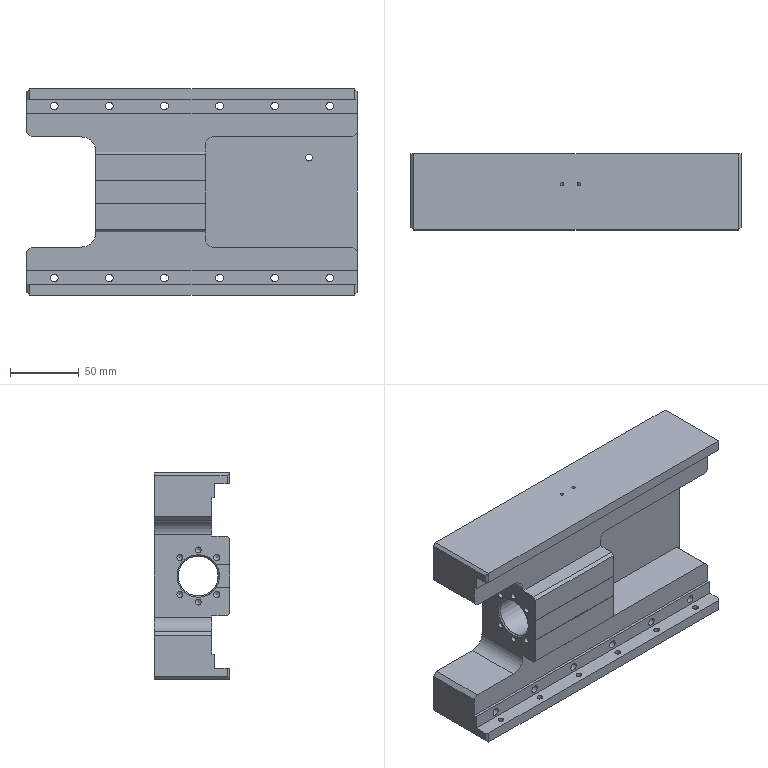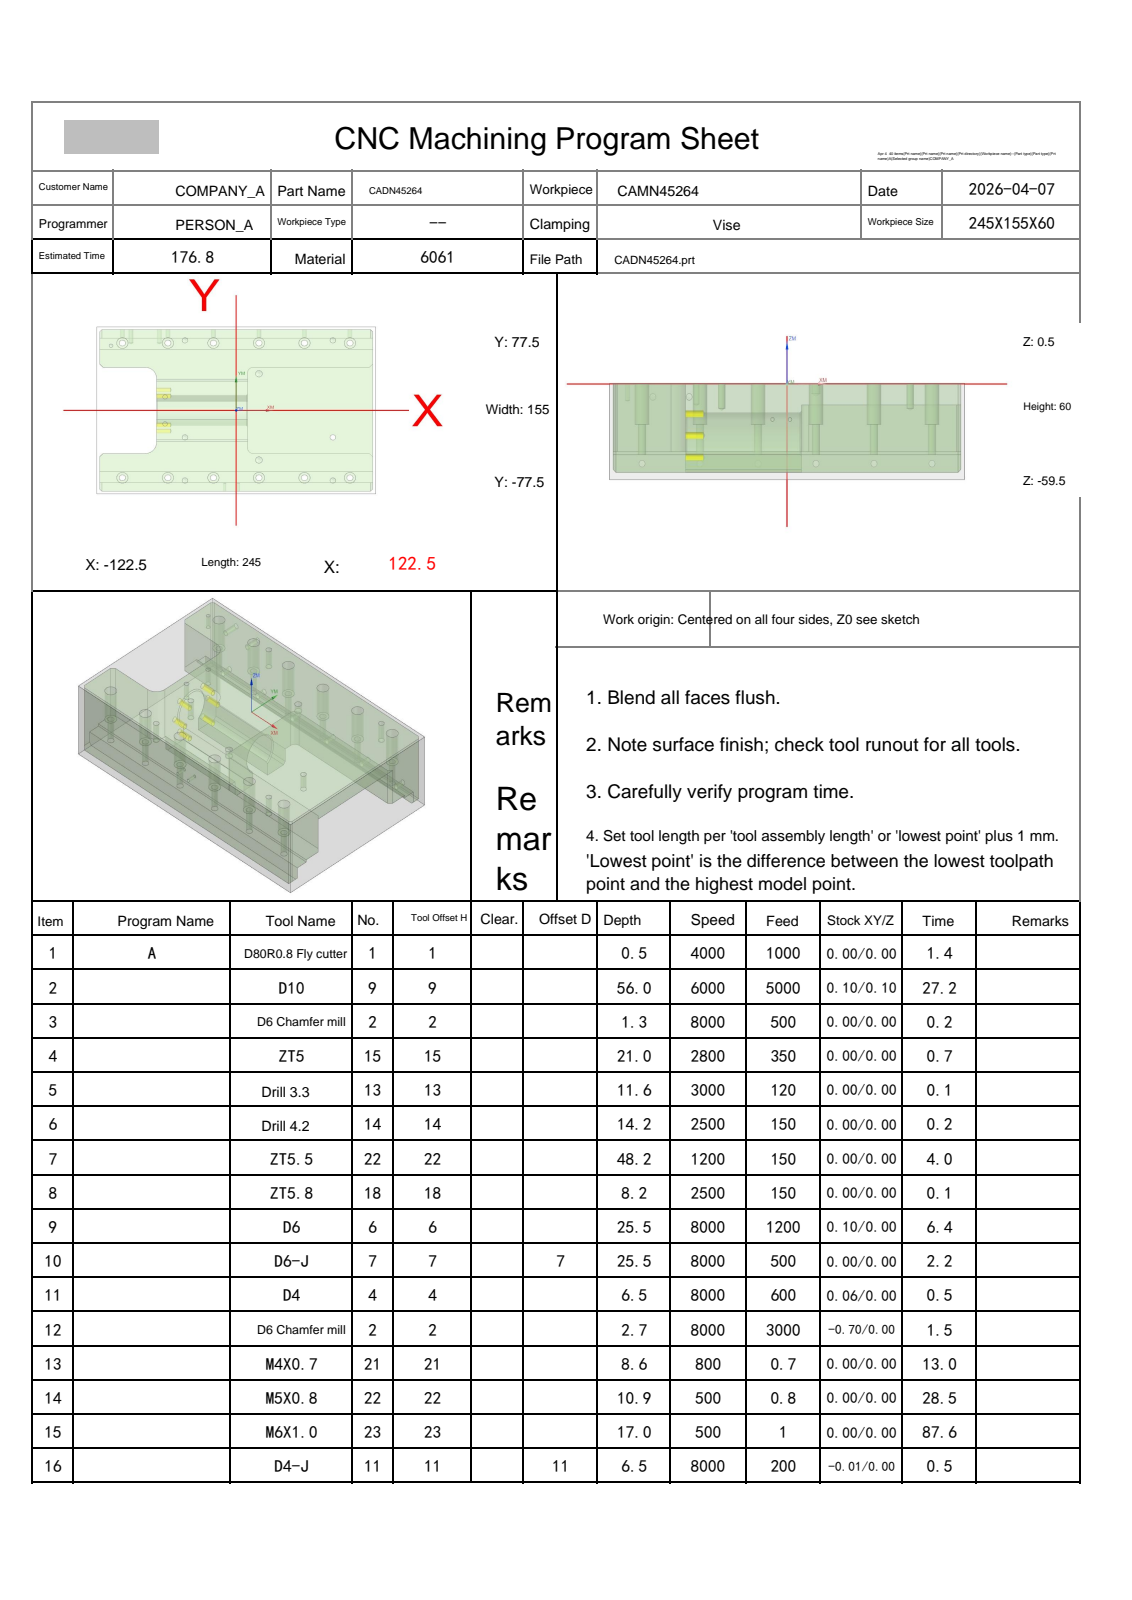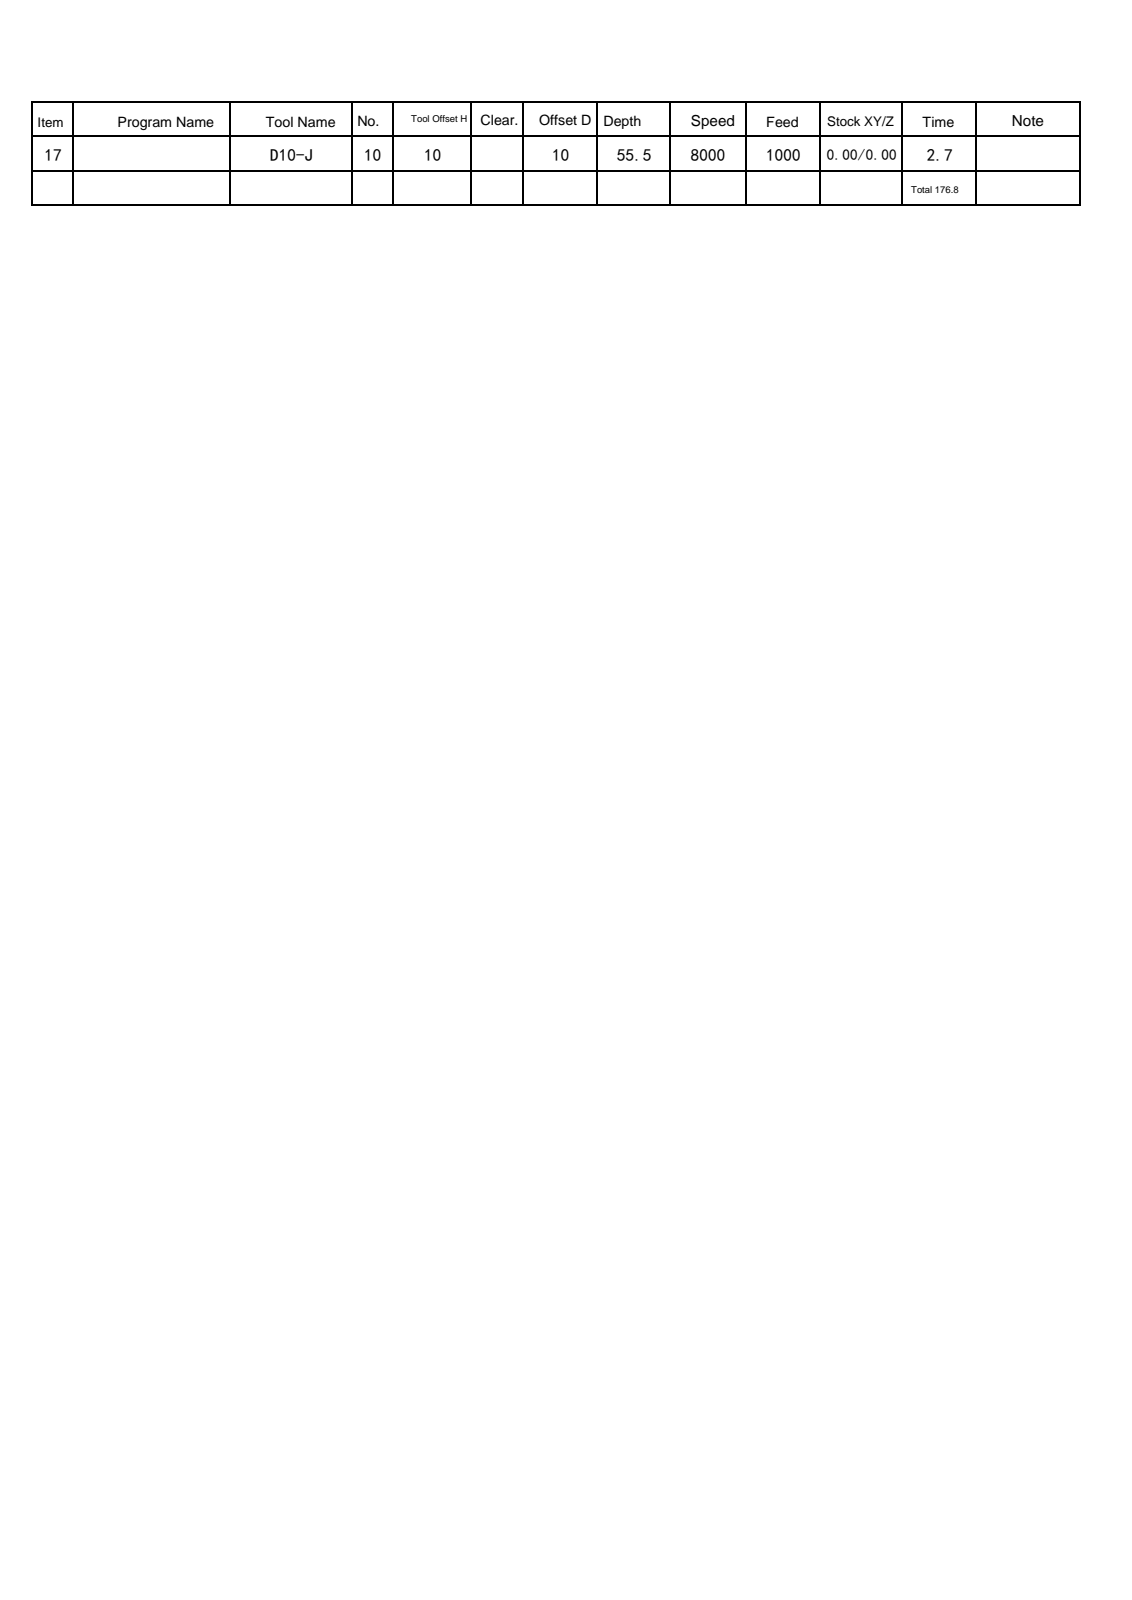NC program | NX | posted by the shop | part box 240 x 55 x 150 mm
Lines 48 to 1046 of 12612:
N2 T09 M06
(D10  D=10. R=0. H=09 ce=0.10 di=0.10)
G00 G90 G54 X-134.5 Y-.734 M03 S6000
G43 H09 Z10.5
M08
Z.603
G01 Z-.597 F5000.
G02 X-129.333 Y1.543 I5.167 J-4.722
X-127.5 Y1.299 I0.0 J-7.
G03 X-123.278 Y.395 I10.5 J38.701
G02 X-122.944 Y0.0 I-.066 J-.395
X-123.278 Y-.395 I-.4 J0.0
G03 X-126.743 Y-1.102 I6.278 J-39.605
X-127.5 Y-2.071 I.243 J-.97
G01 Y-7.652
G03 X-126.8 Y-8.352 I.7 J0.0
X-126.597 Y-8.322 I0.0 J.7
G02 X-117. Y-6.9 I9.597 J-31.678
G01 X-104.096
G03 X-103.1 Y-5.904 I-.004 J1.
G01 Y-2.469
X-103.071 Y-2.414
X-103.13 Y-2.397
X-103.2 Y-2.328
X-103.27 Y-2.296
X-103.247 Y-2.222
G03 X-105.27 Y.1 I-2.496 J-.133
G01 X-119.827 Y2.91
G03 X-120.301 Y2.955 I-.474 J-2.455
X-122.801 Y.455 I0.0 J-2.5
X-120.774 Y-2. I2.5 J0.0
G01 X-106.217 Y-4.81
G03 X-105.743 Y-4.855 I.474 J2.455
X-103.246 Y-2.466 I0.0 J2.5
G01 X-103.216 Y-2.398
X-103.148 Y-2.331
X-103.076 Y-2.293
X-103.1 Y-2.215
Y5.904
G03 X-104.096 Y6.9 I-1. J-.004
G01 X-117.
G02 X-126.796 Y8.383 I0.0 J33.1
X-127.5 Y9.338 I.296 J.955
G01 Y15.203
G02 X-126.9 Y15.803 I.6 J0.0
X-126.678 Y15.761 I0.0 J-.6
G03 X-117. Y13.9 I9.678 J24.239
G01 X-97.096
G02 X-96.1 Y12.904 I-.004 J-1.
G01 Y-12.904
G02 X-97.096 Y-13.9 I-1. J.004
G01 X-117.
G03 X-126.879 Y-15.842 I0.0 J-26.1
X-127.5 Y-16.767 I.379 J-.925
G01 Y-23.143
G03 X-127. Y-23.643 I.5 J0.0
X-126.745 Y-23.573 I0.0 J.5
G02 X-117. Y-20.9 I9.745 J-16.427
G01 X-90.097
G03 X-89.1 Y-19.903 I-.003 J1.
G01 Y19.903
G03 X-90.097 Y20.9 I-1. J-.003
G01 X-117.
G02 X-127.025 Y23.743 I0.0 J19.1
X-127.5 Y24.593 I.525 J.851
G01 Y32.423
G02 X-127.1 Y32.822 I.4 J0.0
X-126.817 Y32.705 I0.0 J-.4
G01 X-125.556 Y31.444
G03 X-117. Y27.9 I8.556 J8.556
G01 X-83.098
G02 X-82.1 Y26.902 I-.002 J-1.
G01 Y-26.902
G02 X-83.098 Y-27.9 I-1. J.002
G01 X-117.
G03 X-125.556 Y-31.444 I0.0 J-12.1
G01 X-126.903 Y-32.791
G03 X-127.195 Y-33.498 I.707 J-.707
X-127.011 Y-34.077 I1. J0.0
G01 X-124.072 Y-38.21
G03 X-123.257 Y-38.631 I.815 J.579
X-122.55 Y-38.338 I0.0 J1.
G01 X-120.606 Y-36.394
G02 X-117. Y-34.9 I3.606 J-3.606
G01 X-80.
G03 X-75.1 Y-30. I0.0 J4.9
G01 Y30.
G03 X-80. Y34.9 I-4.9 J0.0
G01 X-117.
G02 X-120.606 Y36.394 I0.0 J5.1
G01 X-123.606 Y39.394
G02 X-125.1 Y43. I3.606 J3.606
G01 Y73.
G02 X-123.606 Y76.606 I5.1 J0.0
G01 X-121.606 Y78.606
G02 X-118. Y80.1 I3.606 J-3.606
G01 X118.
G02 X121.606 Y78.606 I0.0 J-5.1
G01 X123.606 Y76.606
G02 X125.1 Y73. I-3.606 J-3.606
G01 Y-73.
G02 X123.606 Y-76.606 I-5.1 J0.0
G01 X121.606 Y-78.606
G02 X118. Y-80.1 I-3.606 J3.606
G01 X-118.
G02 X-121.606 Y-78.606 I0.0 J5.1
G01 X-123.606 Y-76.606
G02 X-125.1 Y-73. I3.606 J3.606
G01 Y-43.
G02 X-123.606 Y-39.394 I5.1 J0.0
G01 X-120.606 Y-36.394
G02 X-118.72 Y-35.199 I3.606 J-3.606
X-118.242 Y-35.054 I1.72 J-4.801
G03 X-112.947 Y-28.264 I-1.705 J6.789
X-113.158 Y-26.559 I-7. J0.0
G01 Z.603
G00 Z3.
G01 X-134.5 Y-.734 F6000.
G00 Z.006
G01 Z-1.194 F5000.
G02 X-129.333 Y1.543 I5.167 J-4.722
X-127.5 Y1.299 I0.0 J-7.
G03 X-123.279 Y.395 I10.5 J38.701
G02 X-122.944 Y0.0 I-.066 J-.395
X-123.279 Y-.395 I-.4 J0.0
G03 X-126.743 Y-1.102 I6.279 J-39.605
X-127.5 Y-2.071 I.243 J-.97
G01 Y-7.652
G03 X-126.8 Y-8.352 I.7 J0.0
X-126.597 Y-8.322 I0.0 J.7
G02 X-117. Y-6.9 I9.597 J-31.678
G01 X-104.096
G03 X-103.1 Y-5.904 I-.004 J1.
G01 Y-2.469
X-103.071 Y-2.414
X-103.13 Y-2.397
X-103.2 Y-2.328
X-103.27 Y-2.295
X-103.247 Y-2.222
G03 X-105.27 Y.1 I-2.496 J-.133
G01 X-119.827 Y2.91
G03 X-120.301 Y2.955 I-.474 J-2.455
X-122.801 Y.455 I0.0 J-2.5
X-120.774 Y-2. I2.5 J0.0
G01 X-106.217 Y-4.81
G03 X-105.743 Y-4.855 I.474 J2.455
X-103.246 Y-2.466 I0.0 J2.5
G01 X-103.216 Y-2.398
X-103.148 Y-2.331
X-103.076 Y-2.293
X-103.1 Y-2.215
Y5.904
G03 X-104.096 Y6.9 I-1. J-.004
G01 X-117.
G02 X-126.796 Y8.383 I0.0 J33.1
X-127.5 Y9.338 I.296 J.955
G01 Y15.203
G02 X-126.9 Y15.803 I.6 J0.0
X-126.678 Y15.761 I0.0 J-.6
G03 X-117. Y13.9 I9.678 J24.239
G01 X-97.097
G02 X-96.1 Y12.903 I-.003 J-1.
G01 Y-12.903
G02 X-97.097 Y-13.9 I-1. J.003
G01 X-117.
G03 X-126.879 Y-15.842 I0.0 J-26.1
X-127.5 Y-16.767 I.379 J-.925
G01 Y-23.143
G03 X-127. Y-23.643 I.5 J0.0
X-126.745 Y-23.573 I0.0 J.5
G02 X-117. Y-20.9 I9.745 J-16.427
G01 X-90.098
G03 X-89.1 Y-19.902 I-.002 J1.
G01 Y19.902
G03 X-90.098 Y20.9 I-1. J-.002
G01 X-117.
G02 X-127.025 Y23.743 I0.0 J19.1
X-127.5 Y24.593 I.525 J.851
G01 Y32.423
G02 X-127.1 Y32.822 I.4 J0.0
X-126.817 Y32.705 I0.0 J-.4
G01 X-125.556 Y31.444
G03 X-117. Y27.9 I8.556 J8.556
G01 X-83.099
G02 X-82.1 Y26.901 I-.001 J-1.
G01 Y-26.901
G02 X-83.099 Y-27.9 I-1. J.001
G01 X-117.
G03 X-125.556 Y-31.444 I0.0 J-12.1
G01 X-126.903 Y-32.791
G03 X-127.195 Y-33.498 I.707 J-.707
X-127.011 Y-34.077 I1. J0.0
G01 X-124.072 Y-38.21
G03 X-123.257 Y-38.631 I.815 J.579
X-122.55 Y-38.338 I0.0 J1.
G01 X-120.606 Y-36.394
G02 X-117. Y-34.9 I3.606 J-3.606
G01 X-80.
G03 X-75.1 Y-30. I0.0 J4.9
G01 Y30.
G03 X-80. Y34.9 I-4.9 J0.0
G01 X-117.
G02 X-120.606 Y36.394 I0.0 J5.1
G01 X-123.606 Y39.394
G02 X-125.1 Y43. I3.606 J3.606
G01 Y73.
G02 X-123.606 Y76.606 I5.1 J0.0
G01 X-121.606 Y78.606
G02 X-118. Y80.1 I3.606 J-3.606
G01 X118.
G02 X121.606 Y78.606 I0.0 J-5.1
G01 X123.606 Y76.606
G02 X125.1 Y73. I-3.606 J-3.606
G01 Y-73.
G02 X123.606 Y-76.606 I-5.1 J0.0
G01 X121.606 Y-78.606
G02 X118. Y-80.1 I-3.606 J3.606
G01 X-118.
G02 X-121.606 Y-78.606 I0.0 J5.1
G01 X-123.606 Y-76.606
G02 X-125.1 Y-73. I3.606 J3.606
G01 Y-43.
G02 X-123.606 Y-39.394 I5.1 J0.0
G01 X-120.606 Y-36.394
G02 X-118.72 Y-35.199 I3.606 J-3.606
X-118.242 Y-35.054 I1.72 J-4.801
G03 X-112.947 Y-28.264 I-1.705 J6.789
X-113.158 Y-26.559 I-7. J0.0
G01 Z.006
G00 Z2.403
G01 X-134.5 Y-.734 F6000.
G00 Z-.591
G01 Z-1.791 F5000.
G02 X-129.333 Y1.543 I5.167 J-4.722
X-127.5 Y1.299 I0.0 J-7.
G03 X-123.278 Y.395 I10.5 J38.701
G02 X-122.944 Y0.0 I-.066 J-.395
X-123.278 Y-.395 I-.4 J0.0
G03 X-126.743 Y-1.102 I6.278 J-39.605
X-127.5 Y-2.071 I.243 J-.97
G01 Y-7.652
G03 X-126.8 Y-8.352 I.7 J0.0
X-126.597 Y-8.322 I0.0 J.7
G02 X-117. Y-6.9 I9.597 J-31.678
G01 X-104.096
G03 X-103.1 Y-5.904 I-.004 J1.
G01 Y-2.469
X-103.071 Y-2.414
X-103.13 Y-2.397
X-103.2 Y-2.328
X-103.27 Y-2.296
X-103.247 Y-2.222
G03 X-105.27 Y.1 I-2.496 J-.133
G01 X-119.827 Y2.91
G03 X-120.301 Y2.955 I-.474 J-2.455
X-122.801 Y.455 I0.0 J-2.5
X-120.774 Y-2. I2.5 J0.0
G01 X-106.217 Y-4.81
G03 X-105.743 Y-4.855 I.474 J2.455
X-103.246 Y-2.466 I0.0 J2.5
G01 X-103.216 Y-2.398
X-103.148 Y-2.331
X-103.076 Y-2.293
X-103.1 Y-2.215
Y5.904
G03 X-104.096 Y6.9 I-1. J-.004
G01 X-117.
G02 X-126.796 Y8.383 I0.0 J33.1
X-127.5 Y9.338 I.296 J.955
G01 Y15.203
G02 X-126.9 Y15.803 I.6 J0.0
X-126.678 Y15.761 I0.0 J-.6
G03 X-117. Y13.9 I9.678 J24.239
G01 X-97.096
G02 X-96.1 Y12.904 I-.004 J-1.
G01 Y-12.904
G02 X-97.096 Y-13.9 I-1. J.004
G01 X-117.
G03 X-126.879 Y-15.842 I0.0 J-26.1
X-127.5 Y-16.767 I.379 J-.925
G01 Y-23.143
G03 X-127. Y-23.643 I.5 J0.0
X-126.745 Y-23.573 I0.0 J.5
G02 X-117. Y-20.9 I9.745 J-16.427
G01 X-90.097
G03 X-89.1 Y-19.903 I-.003 J1.
G01 Y19.903
G03 X-90.097 Y20.9 I-1. J-.003
G01 X-117.
G02 X-127.025 Y23.743 I0.0 J19.1
X-127.5 Y24.593 I.525 J.851
G01 Y32.423
G02 X-127.1 Y32.822 I.4 J0.0
X-126.817 Y32.705 I0.0 J-.4
G01 X-125.556 Y31.444
G03 X-117. Y27.9 I8.556 J8.556
G01 X-83.098
G02 X-82.1 Y26.902 I-.002 J-1.
G01 Y-26.902
G02 X-83.098 Y-27.9 I-1. J.002
G01 X-117.
G03 X-125.556 Y-31.444 I0.0 J-12.1
G01 X-126.903 Y-32.791
G03 X-127.195 Y-33.498 I.707 J-.707
X-127.011 Y-34.077 I1. J0.0
G01 X-124.072 Y-38.21
G03 X-123.257 Y-38.631 I.815 J.579
X-122.55 Y-38.338 I0.0 J1.
G01 X-120.606 Y-36.394
G02 X-117. Y-34.9 I3.606 J-3.606
G01 X-80.
G03 X-75.1 Y-30. I0.0 J4.9
G01 Y30.
G03 X-80. Y34.9 I-4.9 J0.0
G01 X-117.
G02 X-120.606 Y36.394 I0.0 J5.1
G01 X-123.606 Y39.394
G02 X-125.1 Y43. I3.606 J3.606
G01 Y73.
G02 X-123.606 Y76.606 I5.1 J0.0
G01 X-121.606 Y78.606
G02 X-118. Y80.1 I3.606 J-3.606
G01 X118.
G02 X121.606 Y78.606 I0.0 J-5.1
G01 X123.606 Y76.606
G02 X125.1 Y73. I-3.606 J-3.606
G01 Y-73.
G02 X123.606 Y-76.606 I-5.1 J0.0
G01 X121.606 Y-78.606
G02 X118. Y-80.1 I-3.606 J3.606
G01 X-118.
G02 X-121.606 Y-78.606 I0.0 J5.1
G01 X-123.606 Y-76.606
G02 X-125.1 Y-73. I3.606 J3.606
G01 Y-43.
G02 X-123.606 Y-39.394 I5.1 J0.0
G01 X-120.606 Y-36.394
G02 X-118.72 Y-35.199 I3.606 J-3.606
X-118.242 Y-35.054 I1.72 J-4.801
G03 X-112.947 Y-28.264 I-1.705 J6.789
X-113.158 Y-26.559 I-7. J0.0
G01 Z-.591
G00 Z1.806
G01 X-134.5 Y-.734 F6000.
G00 Z-1.188
G01 Z-2.388 F5000.
G02 X-129.333 Y1.543 I5.167 J-4.722
X-127.5 Y1.299 I0.0 J-7.
G03 X-123.279 Y.395 I10.5 J38.701
G02 X-122.944 Y0.0 I-.066 J-.395
X-123.279 Y-.395 I-.4 J0.0
G03 X-126.743 Y-1.102 I6.279 J-39.605
X-127.5 Y-2.071 I.243 J-.97
G01 Y-7.652
G03 X-126.8 Y-8.352 I.7 J0.0
X-126.597 Y-8.322 I0.0 J.7
G02 X-117. Y-6.9 I9.597 J-31.678
G01 X-104.096
G03 X-103.1 Y-5.904 I-.004 J1.
G01 Y-2.469
X-103.071 Y-2.414
X-103.13 Y-2.397
X-103.2 Y-2.328
X-103.27 Y-2.295
X-103.247 Y-2.222
G03 X-105.27 Y.1 I-2.496 J-.133
G01 X-119.827 Y2.91
G03 X-120.301 Y2.955 I-.474 J-2.455
X-122.801 Y.455 I0.0 J-2.5
X-120.774 Y-2. I2.5 J0.0
G01 X-106.217 Y-4.81
G03 X-105.743 Y-4.855 I.474 J2.455
X-103.246 Y-2.466 I0.0 J2.5
G01 X-103.216 Y-2.398
X-103.148 Y-2.331
X-103.076 Y-2.293
X-103.1 Y-2.215
Y5.904
G03 X-104.096 Y6.9 I-1. J-.004
G01 X-117.
G02 X-126.796 Y8.383 I0.0 J33.1
X-127.5 Y9.338 I.296 J.955
G01 Y15.203
G02 X-126.9 Y15.803 I.6 J0.0
X-126.678 Y15.761 I0.0 J-.6
G03 X-117. Y13.9 I9.678 J24.239
G01 X-97.097
G02 X-96.1 Y12.903 I-.003 J-1.
G01 Y-12.903
G02 X-97.097 Y-13.9 I-1. J.003
G01 X-117.
G03 X-126.879 Y-15.842 I0.0 J-26.1
X-127.5 Y-16.767 I.379 J-.925
G01 Y-23.143
G03 X-127. Y-23.643 I.5 J0.0
X-126.745 Y-23.573 I0.0 J.5
G02 X-117. Y-20.9 I9.745 J-16.427
G01 X-90.098
G03 X-89.1 Y-19.902 I-.002 J1.
G01 Y19.902
G03 X-90.098 Y20.9 I-1. J-.002
G01 X-117.
G02 X-127.025 Y23.743 I0.0 J19.1
X-127.5 Y24.593 I.525 J.851
G01 Y32.423
G02 X-127.1 Y32.822 I.4 J0.0
X-126.817 Y32.705 I0.0 J-.4
G01 X-125.556 Y31.444
G03 X-117. Y27.9 I8.556 J8.556
G01 X-83.099
G02 X-82.1 Y26.901 I-.001 J-1.
G01 Y-26.901
G02 X-83.099 Y-27.9 I-1. J.001
G01 X-117.
G03 X-125.556 Y-31.444 I0.0 J-12.1
G01 X-126.903 Y-32.791
G03 X-127.195 Y-33.498 I.707 J-.707
X-127.011 Y-34.077 I1. J0.0
G01 X-124.072 Y-38.21
G03 X-123.257 Y-38.631 I.815 J.579
X-122.55 Y-38.338 I0.0 J1.
G01 X-120.606 Y-36.394
G02 X-117. Y-34.9 I3.606 J-3.606
G01 X-80.
G03 X-75.1 Y-30. I0.0 J4.9
G01 Y30.
G03 X-80. Y34.9 I-4.9 J0.0
G01 X-117.
G02 X-120.606 Y36.394 I0.0 J5.1
G01 X-123.606 Y39.394
G02 X-125.1 Y43. I3.606 J3.606
G01 Y73.
G02 X-123.606 Y76.606 I5.1 J0.0
G01 X-121.606 Y78.606
G02 X-118. Y80.1 I3.606 J-3.606
G01 X118.
G02 X121.606 Y78.606 I0.0 J-5.1
G01 X123.606 Y76.606
G02 X125.1 Y73. I-3.606 J-3.606
G01 Y-73.
G02 X123.606 Y-76.606 I-5.1 J0.0
G01 X121.606 Y-78.606
G02 X118. Y-80.1 I-3.606 J3.606
G01 X-118.
G02 X-121.606 Y-78.606 I0.0 J5.1
G01 X-123.606 Y-76.606
G02 X-125.1 Y-73. I3.606 J3.606
G01 Y-43.
G02 X-123.606 Y-39.394 I5.1 J0.0
G01 X-120.606 Y-36.394
G02 X-118.72 Y-35.199 I3.606 J-3.606
X-118.242 Y-35.054 I1.72 J-4.801
G03 X-112.947 Y-28.264 I-1.705 J6.789
X-113.158 Y-26.559 I-7. J0.0
G01 Z-1.188
G00 Z1.209
G01 X-134.5 Y-.734 F6000.
G00 Z-1.785
G01 Z-2.985 F5000.
G02 X-129.333 Y1.543 I5.167 J-4.722
X-127.5 Y1.299 I0.0 J-7.
G03 X-123.278 Y.395 I10.5 J38.701
G02 X-122.944 Y0.0 I-.066 J-.395
X-123.278 Y-.395 I-.4 J0.0
G03 X-126.743 Y-1.102 I6.278 J-39.605
X-127.5 Y-2.071 I.243 J-.97
G01 Y-7.652
G03 X-126.8 Y-8.352 I.7 J0.0
X-126.597 Y-8.322 I0.0 J.7
G02 X-117. Y-6.9 I9.597 J-31.678
G01 X-104.096
G03 X-103.1 Y-5.904 I-.004 J1.
G01 Y-2.469
X-103.071 Y-2.414
X-103.13 Y-2.397
X-103.2 Y-2.328
X-103.27 Y-2.296
X-103.247 Y-2.222
G03 X-105.27 Y.1 I-2.496 J-.133
G01 X-119.827 Y2.91
G03 X-120.301 Y2.955 I-.474 J-2.455
X-122.801 Y.455 I0.0 J-2.5
X-120.774 Y-2. I2.5 J0.0
G01 X-106.217 Y-4.81
G03 X-105.743 Y-4.855 I.474 J2.455
X-103.246 Y-2.466 I0.0 J2.5
G01 X-103.216 Y-2.398
X-103.148 Y-2.331
X-103.076 Y-2.293
X-103.1 Y-2.215
Y5.904
G03 X-104.096 Y6.9 I-1. J-.004
G01 X-117.
G02 X-126.796 Y8.383 I0.0 J33.1
X-127.5 Y9.338 I.296 J.955
G01 Y15.203
G02 X-126.9 Y15.803 I.6 J0.0
X-126.678 Y15.761 I0.0 J-.6
G03 X-117. Y13.9 I9.678 J24.239
G01 X-97.096
G02 X-96.1 Y12.904 I-.004 J-1.
G01 Y-12.904
G02 X-97.096 Y-13.9 I-1. J.004
G01 X-117.
G03 X-126.879 Y-15.842 I0.0 J-26.1
X-127.5 Y-16.767 I.379 J-.925
G01 Y-23.143
G03 X-127. Y-23.643 I.5 J0.0
X-126.745 Y-23.573 I0.0 J.5
G02 X-117. Y-20.9 I9.745 J-16.427
G01 X-90.097
G03 X-89.1 Y-19.903 I-.003 J1.
G01 Y19.903
G03 X-90.097 Y20.9 I-1. J-.003
G01 X-117.
G02 X-127.025 Y23.743 I0.0 J19.1
X-127.5 Y24.593 I.525 J.851
G01 Y32.423
G02 X-127.1 Y32.822 I.4 J0.0
X-126.817 Y32.705 I0.0 J-.4
G01 X-125.556 Y31.444
G03 X-117. Y27.9 I8.556 J8.556
G01 X-83.098
G02 X-82.1 Y26.902 I-.002 J-1.
G01 Y-26.902
G02 X-83.098 Y-27.9 I-1. J.002
G01 X-117.
G03 X-125.556 Y-31.444 I0.0 J-12.1
G01 X-126.903 Y-32.791
G03 X-127.195 Y-33.498 I.707 J-.707
X-127.011 Y-34.077 I1. J0.0
G01 X-124.072 Y-38.21
G03 X-123.257 Y-38.631 I.815 J.579
X-122.55 Y-38.338 I0.0 J1.
G01 X-120.606 Y-36.394
G02 X-117. Y-34.9 I3.606 J-3.606
G01 X-80.
G03 X-75.1 Y-30. I0.0 J4.9
G01 Y30.
G03 X-80. Y34.9 I-4.9 J0.0
G01 X-117.
G02 X-120.606 Y36.394 I0.0 J5.1
G01 X-123.606 Y39.394
G02 X-125.1 Y43. I3.606 J3.606
G01 Y73.
G02 X-123.606 Y76.606 I5.1 J0.0
G01 X-121.606 Y78.606
G02 X-118. Y80.1 I3.606 J-3.606
G01 X118.
G02 X121.606 Y78.606 I0.0 J-5.1
G01 X123.606 Y76.606
G02 X125.1 Y73. I-3.606 J-3.606
G01 Y-73.
G02 X123.606 Y-76.606 I-5.1 J0.0
G01 X121.606 Y-78.606
G02 X118. Y-80.1 I-3.606 J3.606
G01 X-118.
G02 X-121.606 Y-78.606 I0.0 J5.1
G01 X-123.606 Y-76.606
G02 X-125.1 Y-73. I3.606 J3.606
G01 Y-43.
G02 X-123.606 Y-39.394 I5.1 J0.0
G01 X-120.606 Y-36.394
G02 X-118.72 Y-35.199 I3.606 J-3.606
X-118.242 Y-35.054 I1.72 J-4.801
G03 X-112.947 Y-28.264 I-1.705 J6.789
X-113.158 Y-26.559 I-7. J0.0
G01 Z-1.785
G00 Z.612
G01 X-134.5 Y-.734 F6000.
G00 Z-2.383
G01 Z-3.583 F5000.
G02 X-129.333 Y1.543 I5.167 J-4.722
X-127.5 Y1.299 I0.0 J-7.
G03 X-123.279 Y.395 I10.5 J38.701
G02 X-122.944 Y0.0 I-.066 J-.395
X-123.279 Y-.395 I-.4 J0.0
G03 X-126.743 Y-1.102 I6.279 J-39.605
X-127.5 Y-2.071 I.243 J-.97
G01 Y-7.652
G03 X-126.8 Y-8.352 I.7 J0.0
X-126.597 Y-8.322 I0.0 J.7
G02 X-117. Y-6.9 I9.597 J-31.678
G01 X-104.096
G03 X-103.1 Y-5.904 I-.004 J1.
G01 Y-2.469
X-103.071 Y-2.414
X-103.13 Y-2.397
X-103.2 Y-2.328
X-103.27 Y-2.295
X-103.247 Y-2.222
G03 X-105.27 Y.1 I-2.496 J-.133
G01 X-119.827 Y2.91
G03 X-120.301 Y2.955 I-.474 J-2.455
X-122.801 Y.455 I0.0 J-2.5
X-120.774 Y-2. I2.5 J0.0
G01 X-106.217 Y-4.81
G03 X-105.743 Y-4.855 I.474 J2.455
X-103.246 Y-2.466 I0.0 J2.5
G01 X-103.216 Y-2.398
X-103.148 Y-2.331
X-103.076 Y-2.293
X-103.1 Y-2.215
Y5.904
G03 X-104.096 Y6.9 I-1. J-.004
G01 X-117.
G02 X-126.796 Y8.383 I0.0 J33.1
X-127.5 Y9.338 I.296 J.955
G01 Y15.203
G02 X-126.9 Y15.803 I.6 J0.0
X-126.678 Y15.761 I0.0 J-.6
G03 X-117. Y13.9 I9.678 J24.239
G01 X-97.097
G02 X-96.1 Y12.903 I-.003 J-1.
G01 Y-12.903
G02 X-97.097 Y-13.9 I-1. J.003
G01 X-117.
G03 X-126.879 Y-15.842 I0.0 J-26.1
X-127.5 Y-16.767 I.379 J-.925
G01 Y-23.143
G03 X-127. Y-23.643 I.5 J0.0
X-126.745 Y-23.573 I0.0 J.5
G02 X-117. Y-20.9 I9.745 J-16.427
G01 X-90.098
G03 X-89.1 Y-19.902 I-.002 J1.
G01 Y19.902
G03 X-90.098 Y20.9 I-1. J-.002
G01 X-117.
G02 X-127.025 Y23.743 I0.0 J19.1
X-127.5 Y24.593 I.525 J.851
G01 Y32.423
G02 X-127.1 Y32.822 I.4 J0.0
X-126.817 Y32.705 I0.0 J-.4
G01 X-125.556 Y31.444
G03 X-117. Y27.9 I8.556 J8.556
G01 X-83.099
G02 X-82.1 Y26.901 I-.001 J-1.
G01 Y-26.901
G02 X-83.099 Y-27.9 I-1. J.001
G01 X-117.
G03 X-125.556 Y-31.444 I0.0 J-12.1
G01 X-126.903 Y-32.791
G03 X-127.195 Y-33.498 I.707 J-.707
X-127.011 Y-34.077 I1. J0.0
G01 X-124.072 Y-38.21
G03 X-123.257 Y-38.631 I.815 J.579
X-122.55 Y-38.338 I0.0 J1.
G01 X-120.606 Y-36.394
G02 X-117. Y-34.9 I3.606 J-3.606
G01 X-80.
G03 X-75.1 Y-30. I0.0 J4.9
G01 Y30.
G03 X-80. Y34.9 I-4.9 J0.0
G01 X-117.
G02 X-120.606 Y36.394 I0.0 J5.1
G01 X-123.606 Y39.394
G02 X-125.1 Y43. I3.606 J3.606
G01 Y73.
G02 X-123.606 Y76.606 I5.1 J0.0
G01 X-121.606 Y78.606
G02 X-118. Y80.1 I3.606 J-3.606
G01 X118.
G02 X121.606 Y78.606 I0.0 J-5.1
G01 X123.606 Y76.606
G02 X125.1 Y73. I-3.606 J-3.606
G01 Y-73.
G02 X123.606 Y-76.606 I-5.1 J0.0
G01 X121.606 Y-78.606
G02 X118. Y-80.1 I-3.606 J3.606
G01 X-118.
G02 X-121.606 Y-78.606 I0.0 J5.1
G01 X-123.606 Y-76.606
G02 X-125.1 Y-73. I3.606 J3.606
G01 Y-43.
G02 X-123.606 Y-39.394 I5.1 J0.0
G01 X-120.606 Y-36.394
G02 X-118.72 Y-35.199 I3.606 J-3.606
X-118.242 Y-35.054 I1.72 J-4.801
G03 X-112.947 Y-28.264 I-1.705 J6.789
X-113.158 Y-26.559 I-7. J0.0
G01 Z-2.383
G00 Z.015
G01 X-134.5 Y-.734 F6000.
G00 Z-2.98
G01 Z-4.18 F5000.
G02 X-129.333 Y1.543 I5.167 J-4.722
X-127.5 Y1.299 I0.0 J-7.
G03 X-123.278 Y.395 I10.5 J38.701
G02 X-122.944 Y0.0 I-.066 J-.395
X-123.278 Y-.395 I-.4 J0.0
G03 X-126.743 Y-1.102 I6.278 J-39.605
X-127.5 Y-2.071 I.243 J-.97
G01 Y-7.652
G03 X-126.8 Y-8.352 I.7 J0.0
X-126.597 Y-8.322 I0.0 J.7
G02 X-117. Y-6.9 I9.597 J-31.678
G01 X-104.096
G03 X-103.1 Y-5.904 I-.004 J1.
G01 Y-2.469
X-103.071 Y-2.414
X-103.13 Y-2.397
X-103.2 Y-2.328
X-103.27 Y-2.296
X-103.247 Y-2.222
G03 X-105.27 Y.1 I-2.496 J-.133
G01 X-119.827 Y2.91
G03 X-120.301 Y2.955 I-.474 J-2.455
X-122.801 Y.455 I0.0 J-2.5
X-120.774 Y-2. I2.5 J0.0
G01 X-106.217 Y-4.81
G03 X-105.743 Y-4.855 I.474 J2.455
X-103.246 Y-2.466 I0.0 J2.5
G01 X-103.216 Y-2.398
X-103.148 Y-2.331
X-103.076 Y-2.293
X-103.1 Y-2.215
Y5.904
G03 X-104.096 Y6.9 I-1. J-.004
G01 X-117.
G02 X-126.796 Y8.383 I0.0 J33.1
X-127.5 Y9.338 I.296 J.955
G01 Y15.203
G02 X-126.9 Y15.803 I.6 J0.0
X-126.678 Y15.761 I0.0 J-.6
G03 X-117. Y13.9 I9.678 J24.239
G01 X-97.096
G02 X-96.1 Y12.904 I-.004 J-1.
G01 Y-12.904
G02 X-97.096 Y-13.9 I-1. J.004
G01 X-117.
G03 X-126.879 Y-15.842 I0.0 J-26.1
X-127.5 Y-16.767 I.379 J-.925
G01 Y-23.143
G03 X-127. Y-23.643 I.5 J0.0
X-126.745 Y-23.573 I0.0 J.5
G02 X-117. Y-20.9 I9.745 J-16.427
G01 X-90.097
G03 X-89.1 Y-19.903 I-.003 J1.
G01 Y19.903
G03 X-90.097 Y20.9 I-1. J-.003
G01 X-117.
G02 X-127.025 Y23.743 I0.0 J19.1
X-127.5 Y24.593 I.525 J.851
G01 Y32.423
G02 X-127.1 Y32.822 I.4 J0.0
X-126.817 Y32.705 I0.0 J-.4
G01 X-125.556 Y31.444
G03 X-117. Y27.9 I8.556 J8.556
G01 X-83.098
G02 X-82.1 Y26.902 I-.002 J-1.
G01 Y-26.902
G02 X-83.098 Y-27.9 I-1. J.002
G01 X-117.
G03 X-125.556 Y-31.444 I0.0 J-12.1
G01 X-126.903 Y-32.791
G03 X-127.195 Y-33.498 I.707 J-.707
X-127.011 Y-34.077 I1. J0.0
G01 X-124.072 Y-38.21
G03 X-123.257 Y-38.631 I.815 J.579
X-122.55 Y-38.338 I0.0 J1.
G01 X-120.606 Y-36.394
G02 X-117. Y-34.9 I3.606 J-3.606
G01 X-80.
G03 X-75.1 Y-30. I0.0 J4.9
G01 Y30.
G03 X-80. Y34.9 I-4.9 J0.0
G01 X-117.
G02 X-120.606 Y36.394 I0.0 J5.1
G01 X-123.606 Y39.394
G02 X-125.1 Y43. I3.606 J3.606
G01 Y73.
G02 X-123.606 Y76.606 I5.1 J0.0
G01 X-121.606 Y78.606
G02 X-118. Y80.1 I3.606 J-3.606
G01 X118.
G02 X121.606 Y78.606 I0.0 J-5.1
G01 X123.606 Y76.606
G02 X125.1 Y73. I-3.606 J-3.606
G01 Y-73.
G02 X123.606 Y-76.606 I-5.1 J0.0
G01 X121.606 Y-78.606
G02 X118. Y-80.1 I-3.606 J3.606
G01 X-118.
G02 X-121.606 Y-78.606 I0.0 J5.1
G01 X-123.606 Y-76.606
G02 X-125.1 Y-73. I3.606 J3.606
G01 Y-43.
G02 X-123.606 Y-39.394 I5.1 J0.0
G01 X-120.606 Y-36.394
G02 X-118.72 Y-35.199 I3.606 J-3.606
X-118.242 Y-35.054 I1.72 J-4.801
G03 X-112.947 Y-28.264 I-1.705 J6.789
X-113.158 Y-26.559 I-7. J0.0
G01 Z-2.98
G00 Z-.583
G01 X-134.5 Y-.734 F6000.
G00 Z-3.577
G01 Z-4.777 F5000.
G02 X-129.333 Y1.543 I5.167 J-4.722
X-127.5 Y1.299 I0.0 J-7.
G03 X-123.279 Y.395 I10.5 J38.701
G02 X-122.944 Y0.0 I-.066 J-.395
X-123.279 Y-.395 I-.4 J0.0
G03 X-126.743 Y-1.102 I6.279 J-39.605
X-127.5 Y-2.071 I.243 J-.97
G01 Y-7.652
G03 X-126.8 Y-8.352 I.7 J0.0
X-126.597 Y-8.322 I0.0 J.7
G02 X-117. Y-6.9 I9.597 J-31.678
G01 X-104.096
G03 X-103.1 Y-5.904 I-.004 J1.
G01 Y-2.469
X-103.071 Y-2.414
X-103.13 Y-2.397
X-103.2 Y-2.328
X-103.27 Y-2.295
X-103.247 Y-2.222
G03 X-105.27 Y.1 I-2.496 J-.133
G01 X-119.827 Y2.91
G03 X-120.301 Y2.955 I-.474 J-2.455
X-122.801 Y.455 I0.0 J-2.5
X-120.774 Y-2. I2.5 J0.0
G01 X-106.217 Y-4.81
G03 X-105.743 Y-4.855 I.474 J2.455
X-103.246 Y-2.466 I0.0 J2.5
G01 X-103.216 Y-2.398
X-103.148 Y-2.331
X-103.076 Y-2.293
X-103.1 Y-2.215
Y5.904
G03 X-104.096 Y6.9 I-1. J-.004
G01 X-117.
G02 X-126.796 Y8.383 I0.0 J33.1
X-127.5 Y9.338 I.296 J.955
G01 Y15.203
G02 X-126.9 Y15.803 I.6 J0.0
X-126.678 Y15.761 I0.0 J-.6
G03 X-117. Y13.9 I9.678 J24.239
G01 X-97.097
G02 X-96.1 Y12.903 I-.003 J-1.
G01 Y-12.903
G02 X-97.097 Y-13.9 I-1. J.003
G01 X-117.
G03 X-126.879 Y-15.842 I0.0 J-26.1
X-127.5 Y-16.767 I.379 J-.925
G01 Y-23.143
G03 X-127. Y-23.643 I.5 J0.0
X-126.745 Y-23.573 I0.0 J.5
G02 X-117. Y-20.9 I9.745 J-16.427
G01 X-90.098
G03 X-89.1 Y-19.902 I-.002 J1.
G01 Y19.902
G03 X-90.098 Y20.9 I-1. J-.002
G01 X-117.
G02 X-127.025 Y23.743 I0.0 J19.1
X-127.5 Y24.593 I.525 J.851
G01 Y32.423
G02 X-127.1 Y32.822 I.4 J0.0
X-126.817 Y32.705 I0.0 J-.4
G01 X-125.556 Y31.444
G03 X-117. Y27.9 I8.556 J8.556
G01 X-83.099
G02 X-82.1 Y26.901 I-.001 J-1.
G01 Y-26.901
G02 X-83.099 Y-27.9 I-1. J.001
G01 X-117.
G03 X-125.556 Y-31.444 I0.0 J-12.1
G01 X-126.903 Y-32.791
G03 X-127.195 Y-33.498 I.707 J-.707
X-127.011 Y-34.077 I1. J0.0
G01 X-124.072 Y-38.21
G03 X-123.257 Y-38.631 I.815 J.579
X-122.55 Y-38.338 I0.0 J1.
G01 X-120.606 Y-36.394
G02 X-117. Y-34.9 I3.606 J-3.606
G01 X-80.
G03 X-75.1 Y-30. I0.0 J4.9
G01 Y30.
G03 X-80. Y34.9 I-4.9 J0.0
G01 X-117.
G02 X-120.606 Y36.394 I0.0 J5.1
G01 X-123.606 Y39.394
G02 X-125.1 Y43. I3.606 J3.606
G01 Y73.
G02 X-123.606 Y76.606 I5.1 J0.0
G01 X-121.606 Y78.606
G02 X-118. Y80.1 I3.606 J-3.606
G01 X118.
G02 X121.606 Y78.606 I0.0 J-5.1
G01 X123.606 Y76.606
G02 X125.1 Y73. I-3.606 J-3.606
G01 Y-73.
G02 X123.606 Y-76.606 I-5.1 J0.0
G01 X121.606 Y-78.606
G02 X118. Y-80.1 I-3.606 J3.606
G01 X-118.
G02 X-121.606 Y-78.606 I0.0 J5.1
G01 X-123.606 Y-76.606
G02 X-125.1 Y-73. I3.606 J3.606
G01 Y-43.
G02 X-123.606 Y-39.394 I5.1 J0.0
G01 X-120.606 Y-36.394
G02 X-118.72 Y-35.199 I3.606 J-3.606
X-118.242 Y-35.054 I1.72 J-4.801
G03 X-112.947 Y-28.264 I-1.705 J6.789
X-113.158 Y-26.559 I-7. J0.0
G01 Z-3.577
G00 Z-1.18
G01 X-134.5 Y-.734 F6000.
G00 Z-4.174
G01 Z-5.374 F5000.
G02 X-129.333 Y1.543 I5.167 J-4.722
X-127.5 Y1.299 I0.0 J-7.
G03 X-123.278 Y.395 I10.5 J38.701
G02 X-122.944 Y0.0 I-.066 J-.395
X-123.278 Y-.395 I-.4 J0.0
G03 X-126.743 Y-1.102 I6.278 J-39.605
X-127.5 Y-2.071 I.243 J-.97
G01 Y-7.652
G03 X-126.8 Y-8.352 I.7 J0.0
X-126.597 Y-8.322 I0.0 J.7
G02 X-117. Y-6.9 I9.597 J-31.678
G01 X-104.096
G03 X-103.1 Y-5.904 I-.004 J1.
G01 Y-2.469
X-103.071 Y-2.414
X-103.13 Y-2.397
X-103.2 Y-2.328
X-103.27 Y-2.296
X-103.247 Y-2.222
G03 X-105.27 Y.1 I-2.496 J-.133
G01 X-119.827 Y2.91
G03 X-120.301 Y2.955 I-.474 J-2.455
X-122.801 Y.455 I0.0 J-2.5
X-120.774 Y-2. I2.5 J0.0
G01 X-106.217 Y-4.81
G03 X-105.743 Y-4.855 I.474 J2.455
X-103.246 Y-2.466 I0.0 J2.5
G01 X-103.216 Y-2.398
X-103.148 Y-2.331
X-103.076 Y-2.293
X-103.1 Y-2.215
Y5.904
G03 X-104.096 Y6.9 I-1. J-.004
G01 X-117.
G02 X-126.796 Y8.383 I0.0 J33.1
X-127.5 Y9.338 I.296 J.955
G01 Y15.203
G02 X-126.9 Y15.803 I.6 J0.0
X-126.678 Y15.761 I0.0 J-.6
G03 X-117. Y13.9 I9.678 J24.239
G01 X-97.096
G02 X-96.1 Y12.904 I-.004 J-1.
G01 Y-12.904
G02 X-97.096 Y-13.9 I-1. J.004
G01 X-117.
G03 X-126.879 Y-15.842 I0.0 J-26.1
X-127.5 Y-16.767 I.379 J-.925
G01 Y-23.143
G03 X-127. Y-23.643 I.5 J0.0
X-126.745 Y-23.573 I0.0 J.5
G02 X-117. Y-20.9 I9.745 J-16.427
G01 X-90.097
G03 X-89.1 Y-19.903 I-.003 J1.
G01 Y19.903
G03 X-90.097 Y20.9 I-1. J-.003
G01 X-117.
G02 X-127.025 Y23.743 I0.0 J19.1
X-127.5 Y24.593 I.525 J.851
G01 Y32.423
G02 X-127.1 Y32.822 I.4 J0.0
X-126.817 Y32.705 I0.0 J-.4
G01 X-125.556 Y31.444
G03 X-117. Y27.9 I8.556 J8.556
G01 X-83.098
G02 X-82.1 Y26.902 I-.002 J-1.
G01 Y-26.902
G02 X-83.098 Y-27.9 I-1. J.002
G01 X-117.
G03 X-125.556 Y-31.444 I0.0 J-12.1
G01 X-126.903 Y-32.791
G03 X-127.195 Y-33.498 I.707 J-.707
X-127.011 Y-34.077 I1. J0.0
G01 X-124.072 Y-38.21
G03 X-123.257 Y-38.631 I.815 J.579
X-122.55 Y-38.338 I0.0 J1.
G01 X-120.606 Y-36.394
G02 X-117. Y-34.9 I3.606 J-3.606
G01 X-80.
G03 X-75.1 Y-30. I0.0 J4.9
G01 Y30.
G03 X-80. Y34.9 I-4.9 J0.0
G01 X-117.
G02 X-120.606 Y36.394 I0.0 J5.1
G01 X-123.606 Y39.394
G02 X-125.1 Y43. I3.606 J3.606
G01 Y73.
G02 X-123.606 Y76.606 I5.1 J0.0
G01 X-121.606 Y78.606